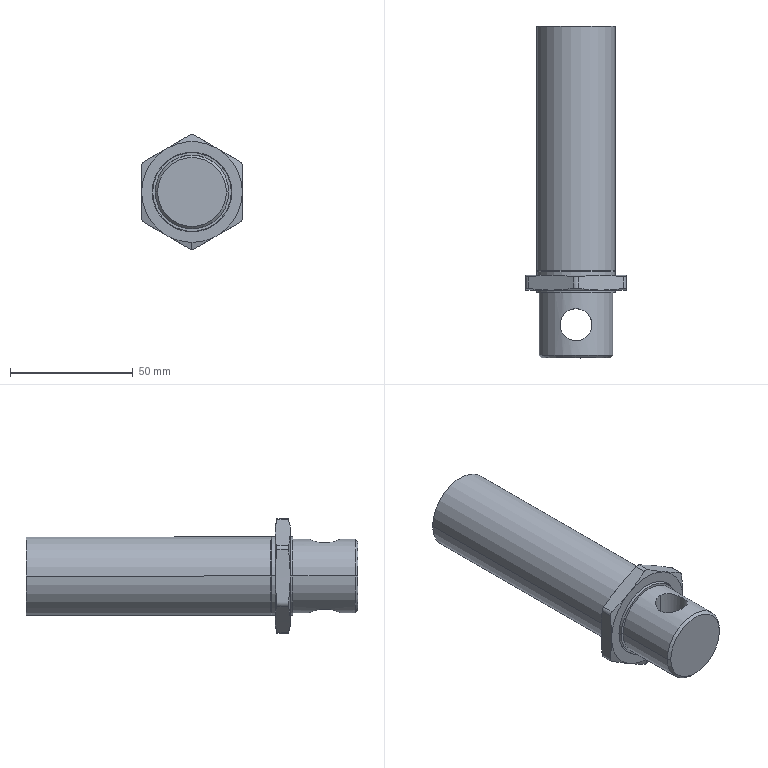Part | SolidWorks | features BaseBody 1 | 1 solid | 57 faces | box 41.006 x 135.111 x 46.725 mm | volume 105123 mm3 | cone 24 | cylinder 20 | plane 13 | commonest cylinder face diameters 4 x8 32 x6 13 x2 18 x2 30 x2